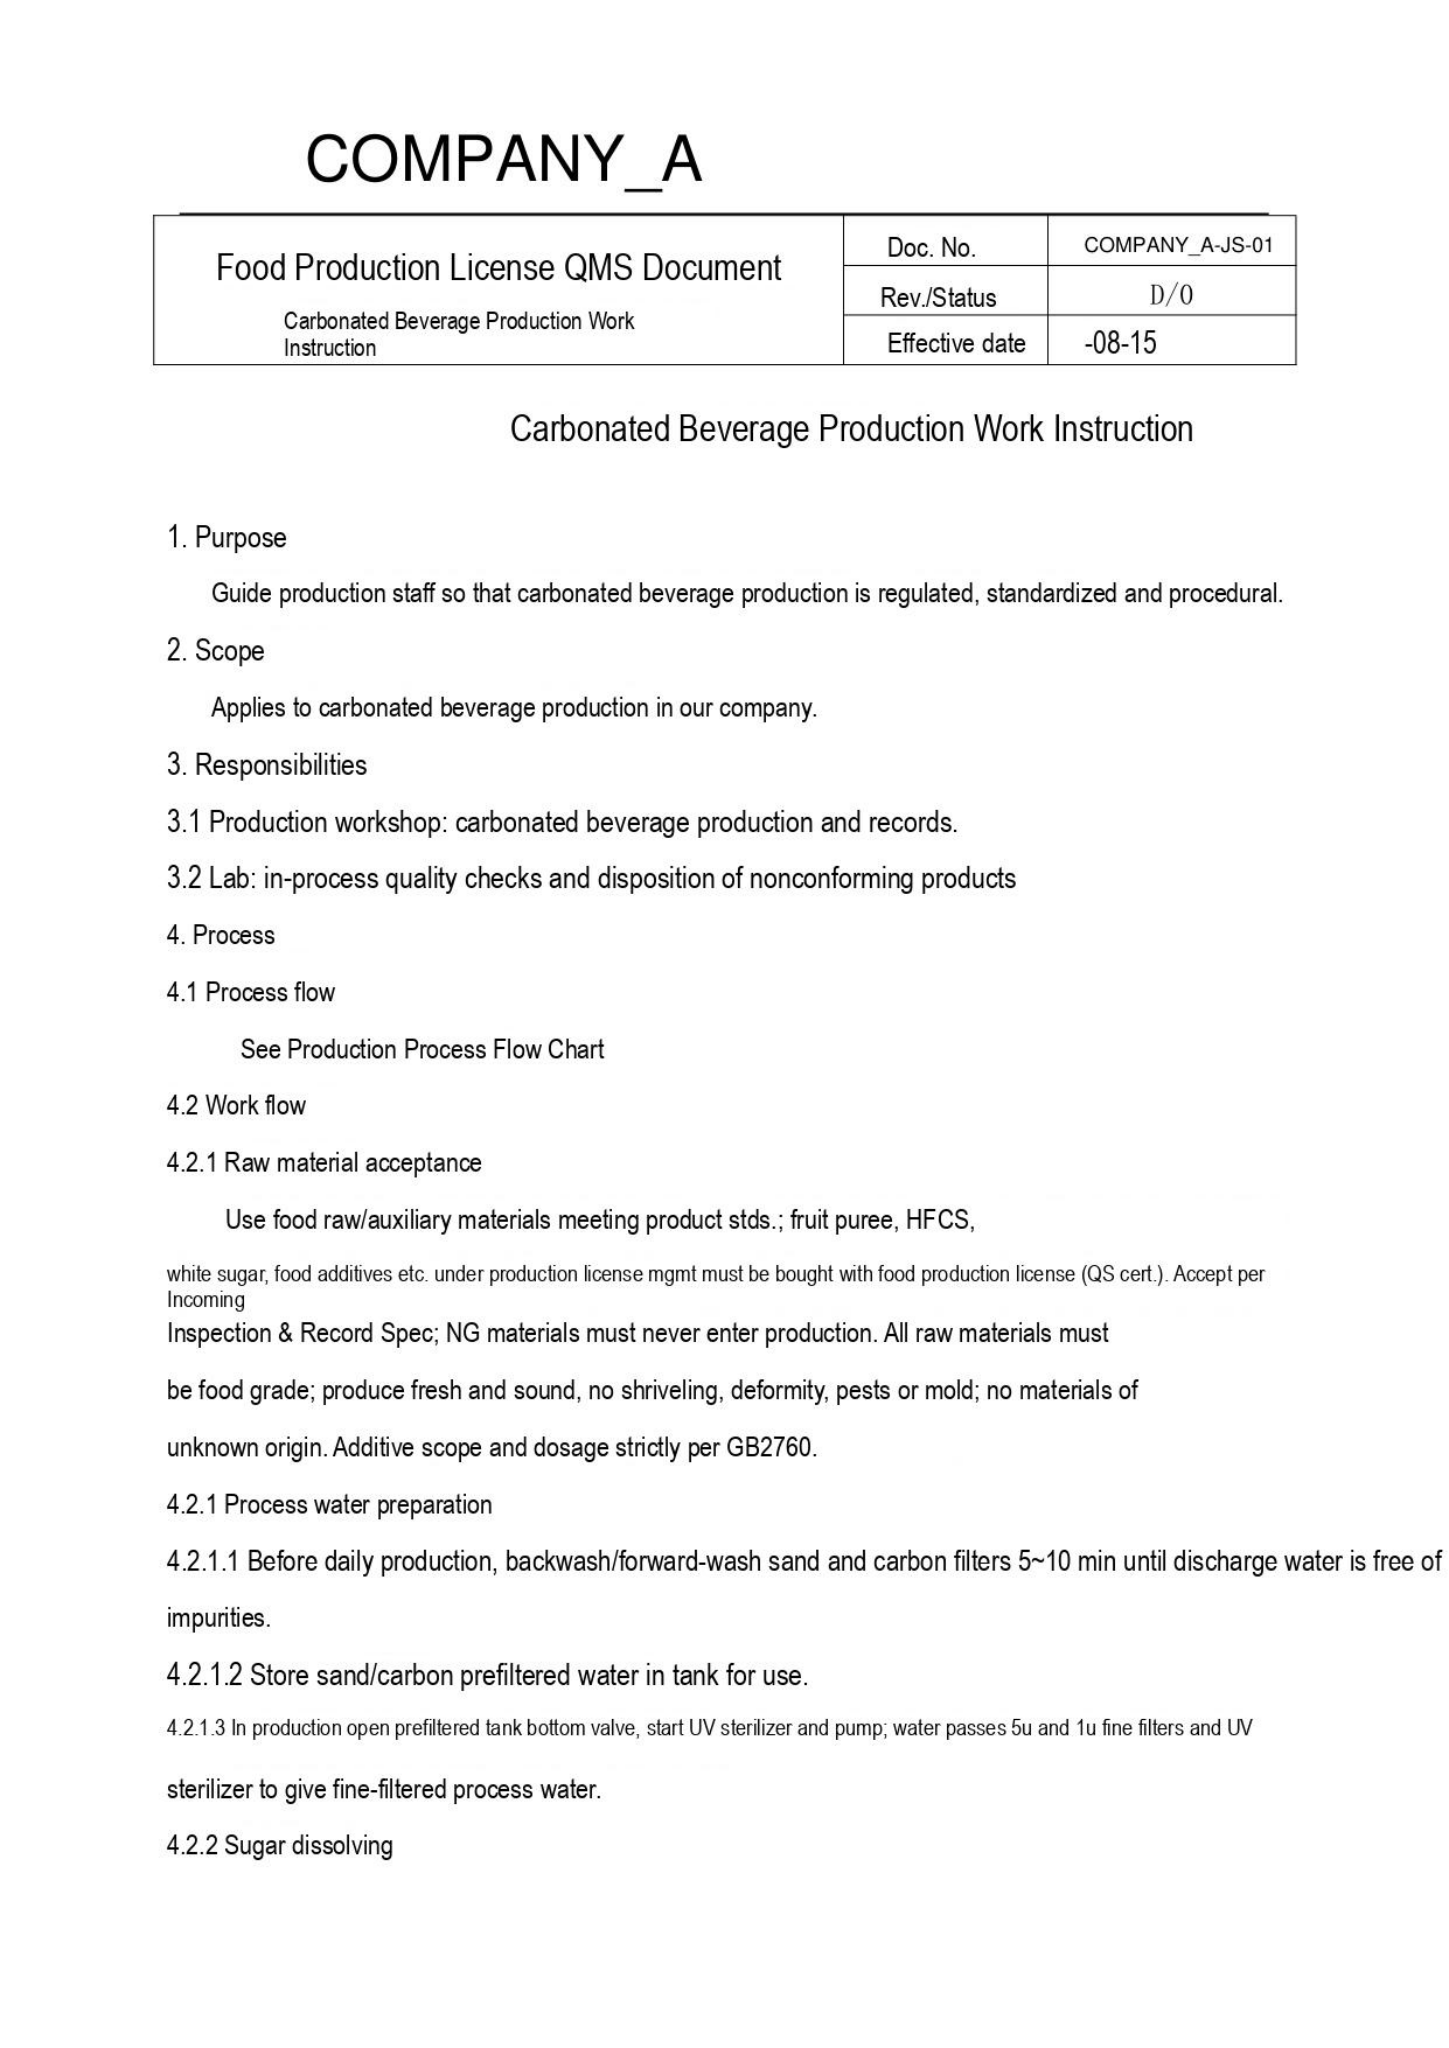COMPANY_A

| Food Production License QMS Document<br>Carbonated Beverage Production Work Instruction | Doc. No. | COMPANY_A-JS-01 |
|---|---|---|
| | Rev./Status | D/0 |
| | Effective date | -08-15 |

Carbonated Beverage Production Work Instruction

1. Purpose

Guide production staff so that carbonated beverage production is regulated, standardized and procedural.

2. Scope

Applies to carbonated beverage production in our company.

3. Responsibilities

3.1 Production workshop: carbonated beverage production and records.

3.2 Lab: in-process quality checks and disposition of nonconforming products

4. Process

4.1 Process flow

See Production Process Flow Chart

4.2 Work flow

4.2.1 Raw material acceptance

Use food raw/auxiliary materials meeting product stds.; fruit puree, HFCS,

white sugar, food additives etc. under production license mgmt must be bought with food production license (QS cert.). Accept per Incoming

Inspection & Record Spec; NG materials must never enter production. All raw materials must

be food grade; produce fresh and sound, no shriveling, deformity, pests or mold; no materials of

unknown origin. Additive scope and dosage strictly per GB2760.

4.2.1 Process water preparation

4.2.1.1 Before daily production, backwash/forward-wash sand and carbon filters 5~10 min until discharge water is free of impurities.

4.2.1.2 Store sand/carbon prefiltered water in tank for use.

4.2.1.3 In production open prefiltered tank bottom valve, start UV sterilizer and pump; water passes 5u and 1u fine filters and UV

sterilizer to give fine-filtered process water.

4.2.2 Sugar dissolving
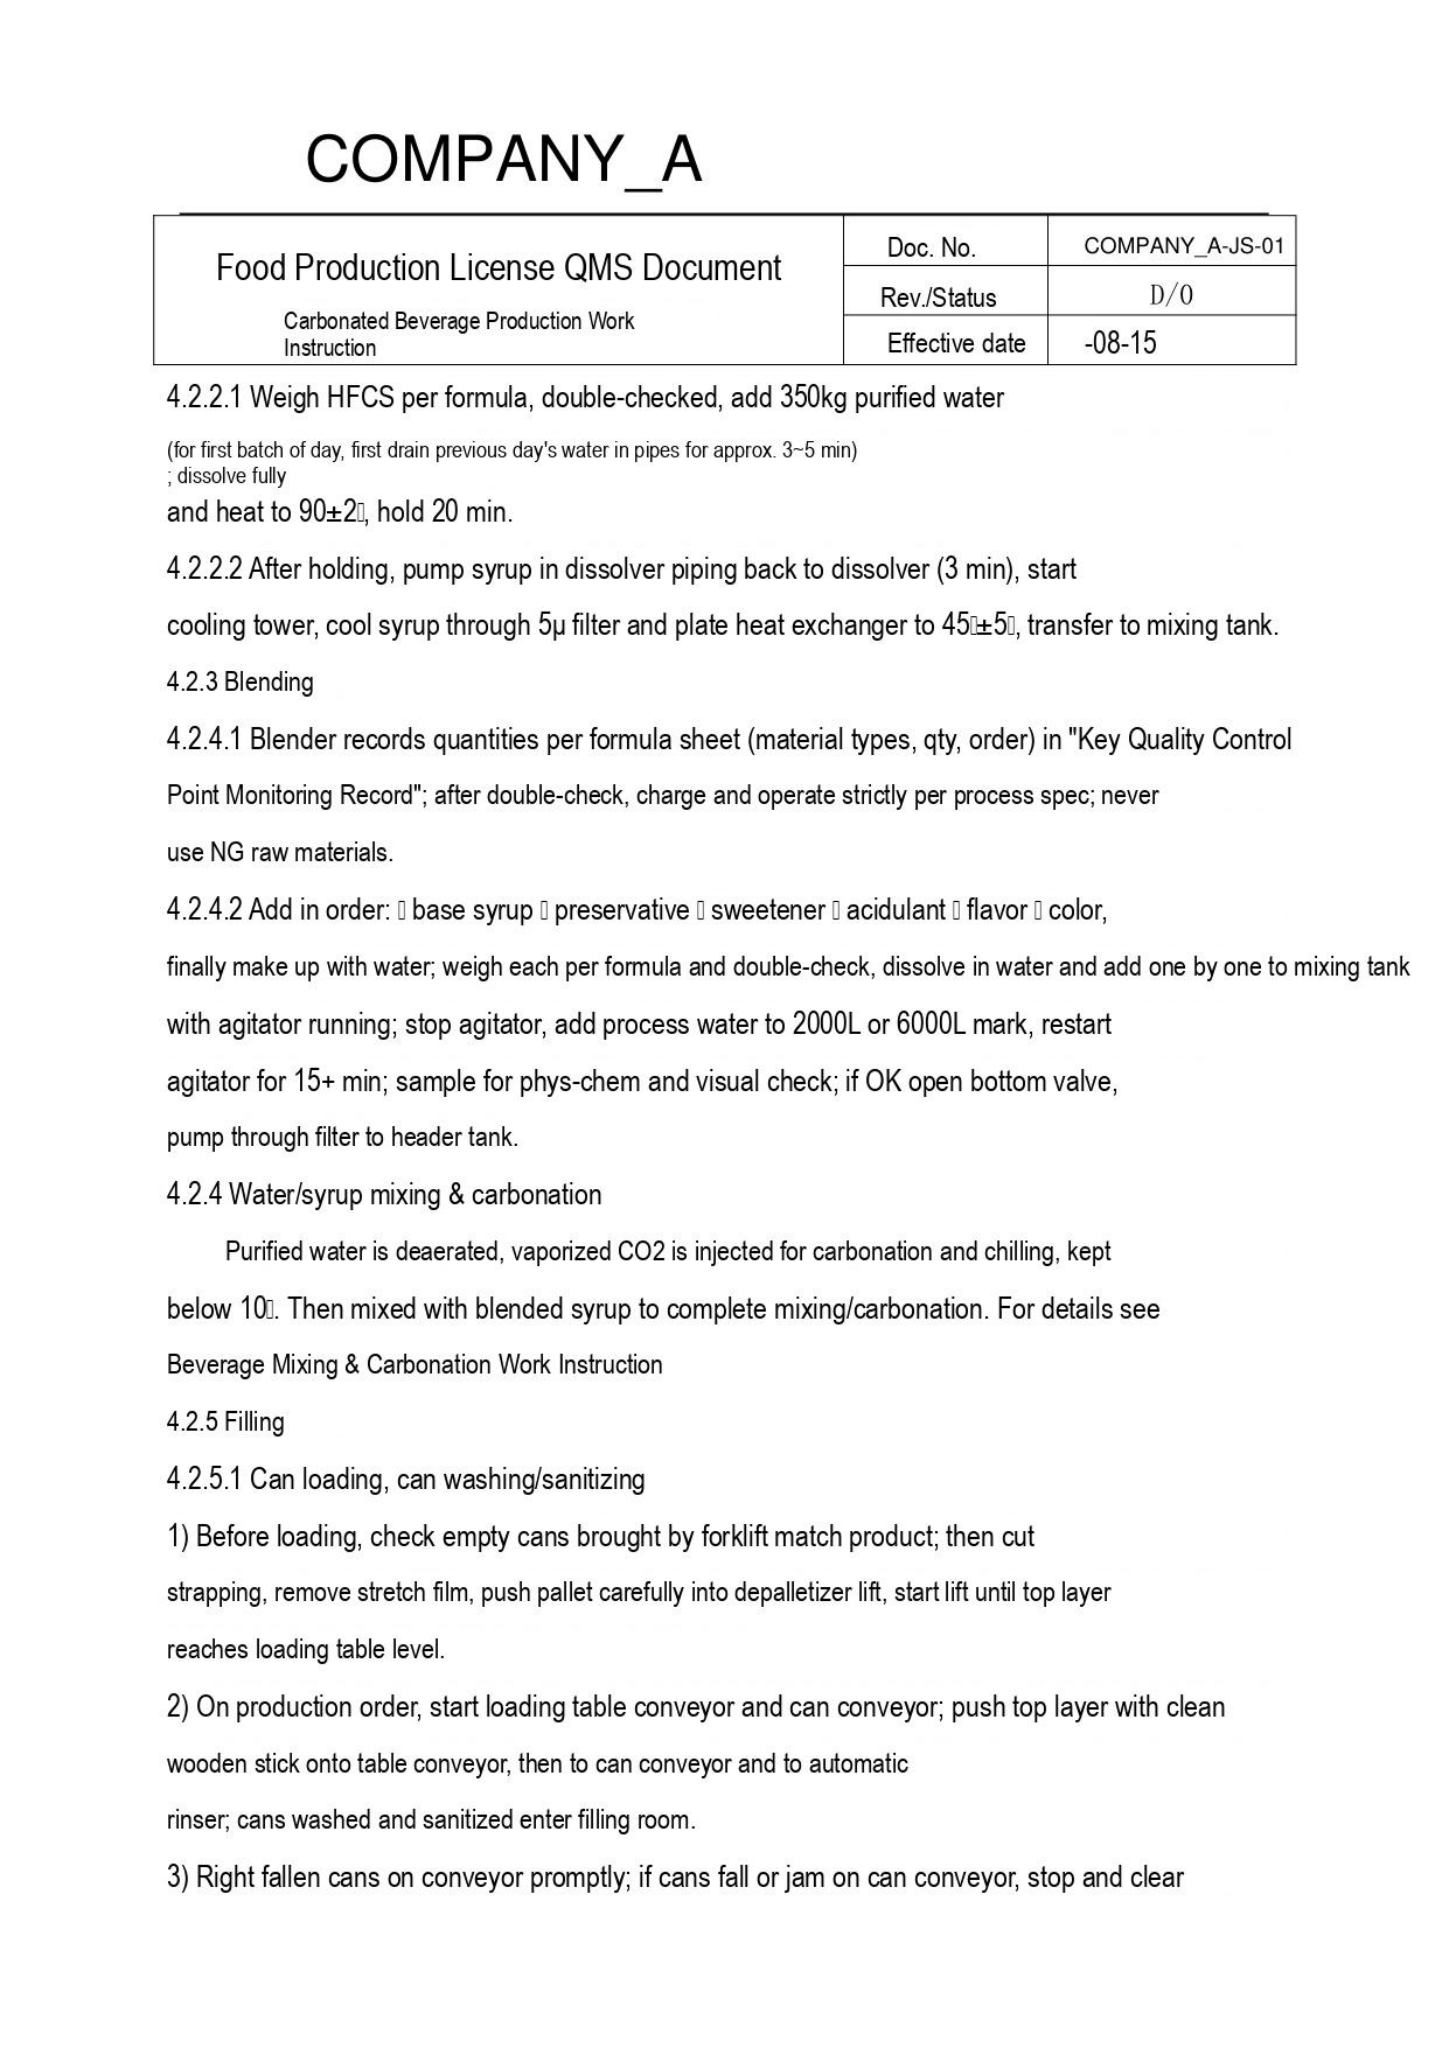COMPANY_A

| Food Production License QMS Document<br>Carbonated Beverage Production Work Instruction | Doc. No. | COMPANY_A-JS-01 |
|---|---|---|
| | Rev./Status | D/0 |
| | Effective date | -08-15 |

4.2.2.1 Weigh HFCS per formula, double-checked, add 350kg purified water

(for first batch of day, first drain previous day's water in pipes for approx. 3~5 min)
; dissolve fully

and heat to 90±2, hold 20 min.

4.2.2.2 After holding, pump syrup in dissolver piping back to dissolver (3 min), start

cooling tower, cool syrup through 5μ filter and plate heat exchanger to 45±5, transfer to mixing tank.

4.2.3 Blending

4.2.4.1 Blender records quantities per formula sheet (material types, qty, order) in "Key Quality Control

Point Monitoring Record"; after double-check, charge and operate strictly per process spec; never

use NG raw materials.

4.2.4.2 Add in order: base syrup preservative sweetener acidulant flavor color,

finally make up with water; weigh each per formula and double-check, dissolve in water and add one by one to mixing tank

with agitator running; stop agitator, add process water to 2000L or 6000L mark, restart

agitator for 15+ min; sample for phys-chem and visual check; if OK open bottom valve,

pump through filter to header tank.

4.2.4 Water/syrup mixing & carbonation

Purified water is deaerated, vaporized CO2 is injected for carbonation and chilling, kept

below 10. Then mixed with blended syrup to complete mixing/carbonation. For details see

Beverage Mixing & Carbonation Work Instruction

4.2.5 Filling

4.2.5.1 Can loading, can washing/sanitizing

1) Before loading, check empty cans brought by forklift match product; then cut

strapping, remove stretch film, push pallet carefully into depalletizer lift, start lift until top layer

reaches loading table level.

2) On production order, start loading table conveyor and can conveyor; push top layer with clean

wooden stick onto table conveyor, then to can conveyor and to automatic

rinser; cans washed and sanitized enter filling room.

3) Right fallen cans on conveyor promptly; if cans fall or jam on can conveyor, stop and clear
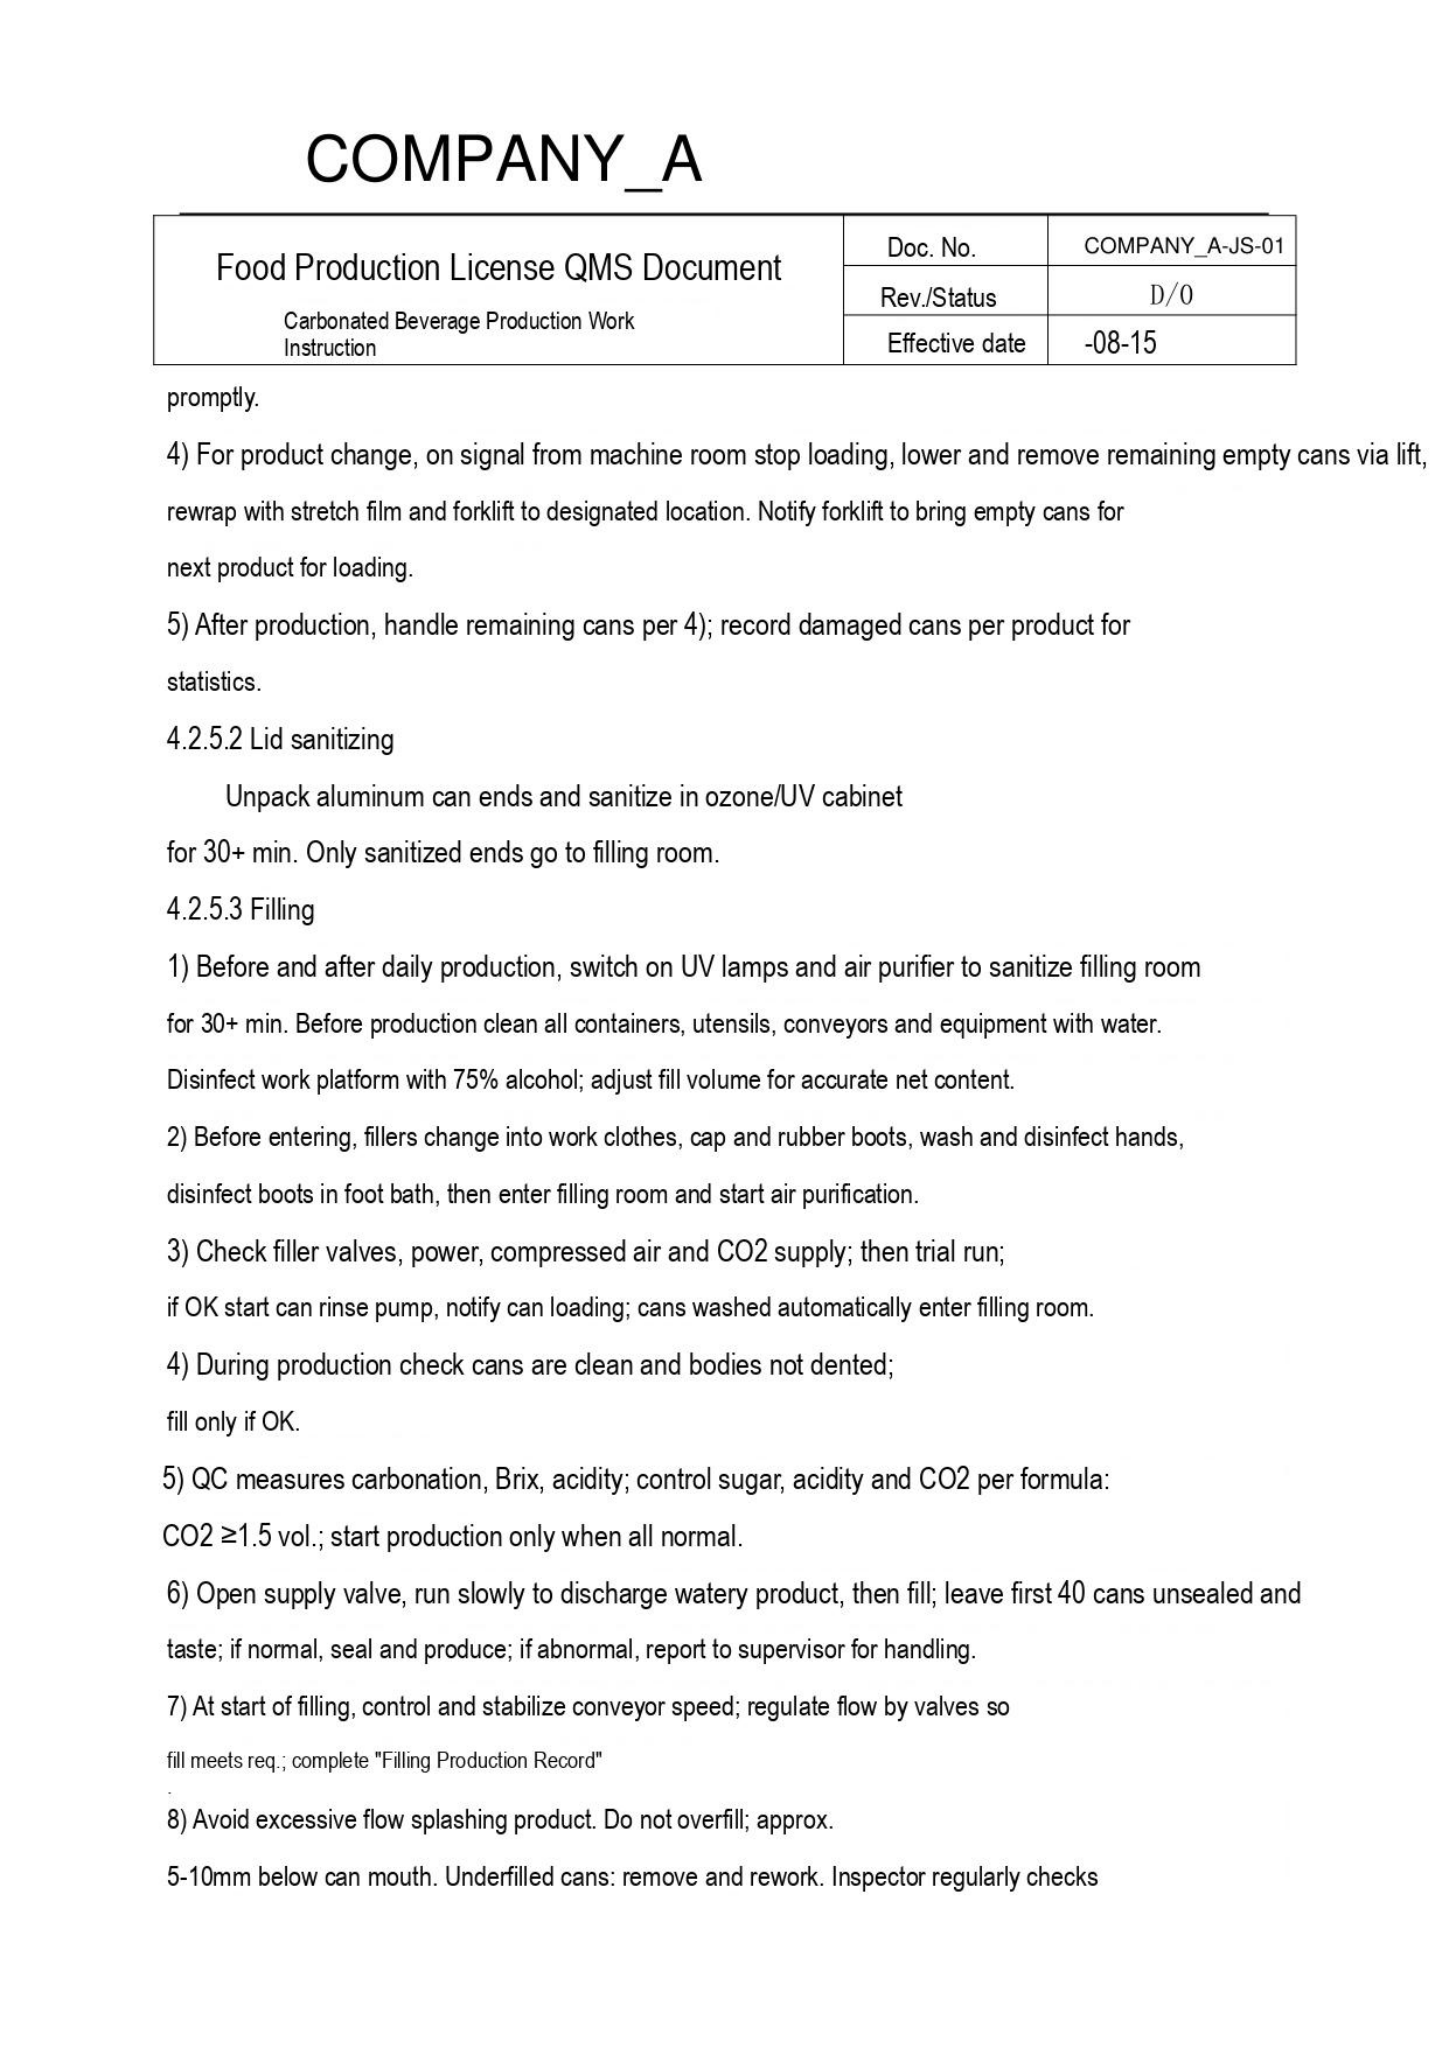COMPANY_A

| Food Production License QMS Document<br>Carbonated Beverage Production Work Instruction | Doc. No. | COMPANY_A-JS-01 |
|---|---|---|
| | Rev./Status | D/0 |
| | Effective date | -08-15 |

promptly.

4) For product change, on signal from machine room stop loading, lower and remove remaining empty cans via lift, rewrap with stretch film and forklift to designated location. Notify forklift to bring empty cans for next product for loading.

5) After production, handle remaining cans per 4); record damaged cans per product for statistics.

4.2.5.2 Lid sanitizing

Unpack aluminum can ends and sanitize in ozone/UV cabinet for 30+ min. Only sanitized ends go to filling room.

4.2.5.3 Filling

1) Before and after daily production, switch on UV lamps and air purifier to sanitize filling room for 30+ min. Before production clean all containers, utensils, conveyors and equipment with water. Disinfect work platform with 75% alcohol; adjust fill volume for accurate net content.

2) Before entering, fillers change into work clothes, cap and rubber boots, wash and disinfect hands, disinfect boots in foot bath, then enter filling room and start air purification.

3) Check filler valves, power, compressed air and CO2 supply; then trial run; if OK start can rinse pump, notify can loading; cans washed automatically enter filling room.

4) During production check cans are clean and bodies not dented; fill only if OK.

5) QC measures carbonation, Brix, acidity; control sugar, acidity and CO2 per formula: CO2 ≥1.5 vol.; start production only when all normal.

6) Open supply valve, run slowly to discharge watery product, then fill; leave first 40 cans unsealed and taste; if normal, seal and produce; if abnormal, report to supervisor for handling.

7) At start of filling, control and stabilize conveyor speed; regulate flow by valves so fill meets req.; complete "Filling Production Record"

8) Avoid excessive flow splashing product. Do not overfill; approx. 5-10mm below can mouth. Underfilled cans: remove and rework. Inspector regularly checks
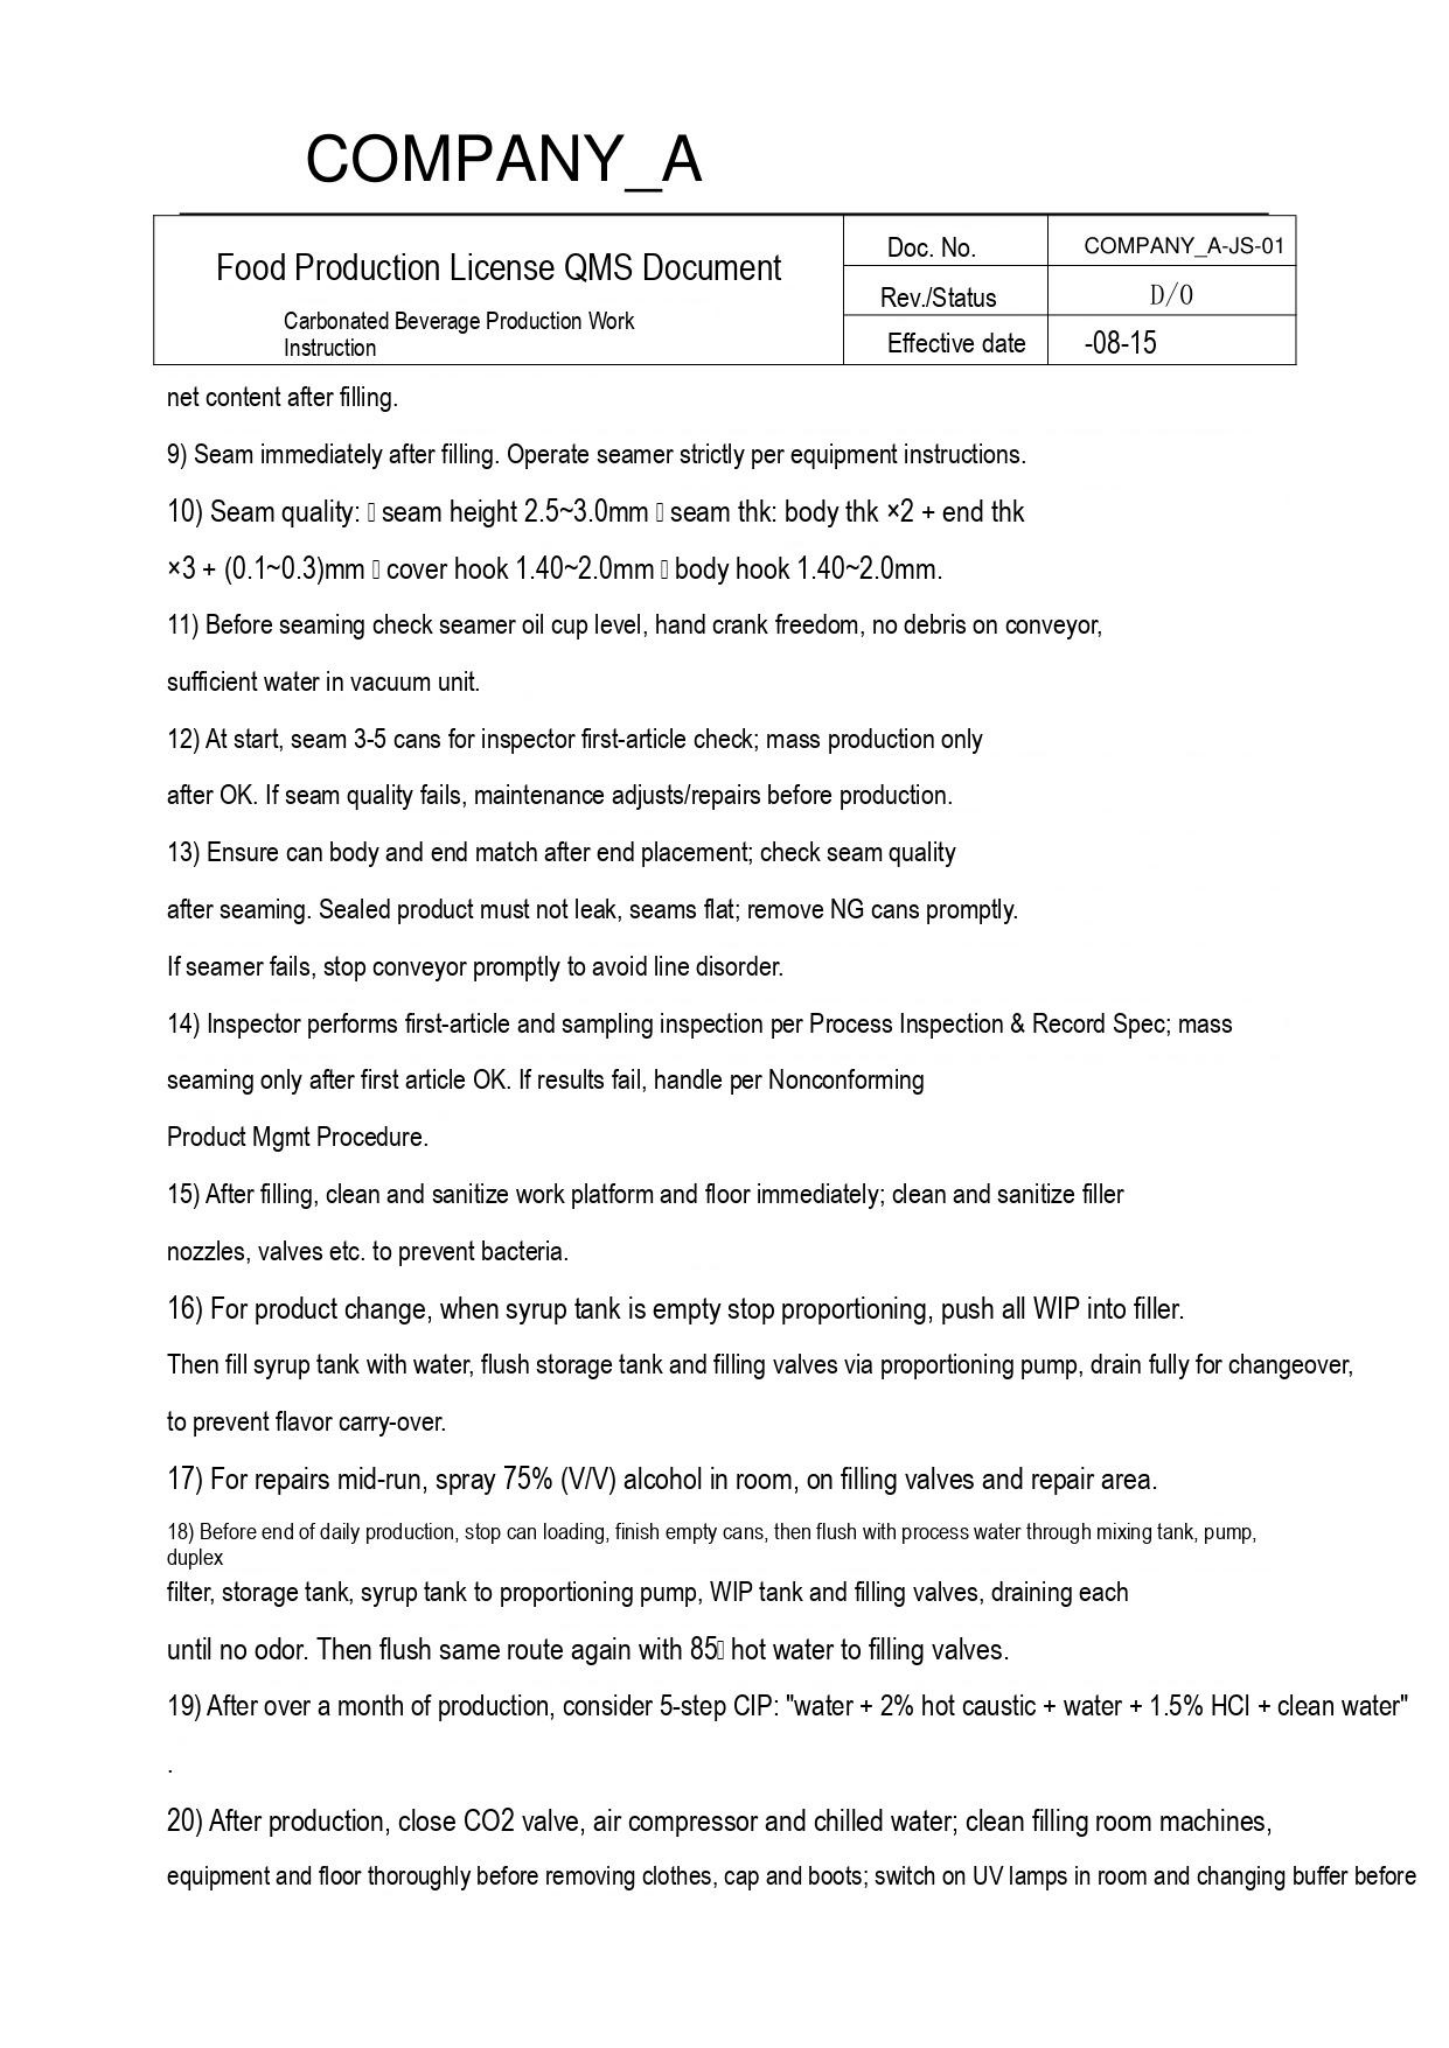COMPANY_A

| Food Production License QMS Document<br>Carbonated Beverage Production Work Instruction | Doc. No. | COMPANY_A-JS-01 |
|---|---|---|
| | Rev./Status | D/0 |
| | Effective date | -08-15 |

net content after filling.

9) Seam immediately after filling. Operate seamer strictly per equipment instructions.

10) Seam quality: seam height 2.5~3.0mm seam thk: body thk ×2 + end thk ×3 + (0.1~0.3)mm cover hook 1.40~2.0mm body hook 1.40~2.0mm.

11) Before seaming check seamer oil cup level, hand crank freedom, no debris on conveyor, sufficient water in vacuum unit.

12) At start, seam 3-5 cans for inspector first-article check; mass production only after OK. If seam quality fails, maintenance adjusts/repairs before production.

13) Ensure can body and end match after end placement; check seam quality after seaming. Sealed product must not leak, seams flat; remove NG cans promptly. If seamer fails, stop conveyor promptly to avoid line disorder.

14) Inspector performs first-article and sampling inspection per Process Inspection & Record Spec; mass seaming only after first article OK. If results fail, handle per Nonconforming Product Mgmt Procedure.

15) After filling, clean and sanitize work platform and floor immediately; clean and sanitize filler nozzles, valves etc. to prevent bacteria.

16) For product change, when syrup tank is empty stop proportioning, push all WIP into filler. Then fill syrup tank with water, flush storage tank and filling valves via proportioning pump, drain fully for changeover, to prevent flavor carry-over.

17) For repairs mid-run, spray 75% (V/V) alcohol in room, on filling valves and repair area.

18) Before end of daily production, stop can loading, finish empty cans, then flush with process water through mixing tank, pump, duplex filter, storage tank, syrup tank to proportioning pump, WIP tank and filling valves, draining each until no odor. Then flush same route again with 85 hot water to filling valves.

19) After over a month of production, consider 5-step CIP: "water + 2% hot caustic + water + 1.5% HCl + clean water".

20) After production, close CO2 valve, air compressor and chilled water; clean filling room machines, equipment and floor thoroughly before removing clothes, cap and boots; switch on UV lamps in room and changing buffer before
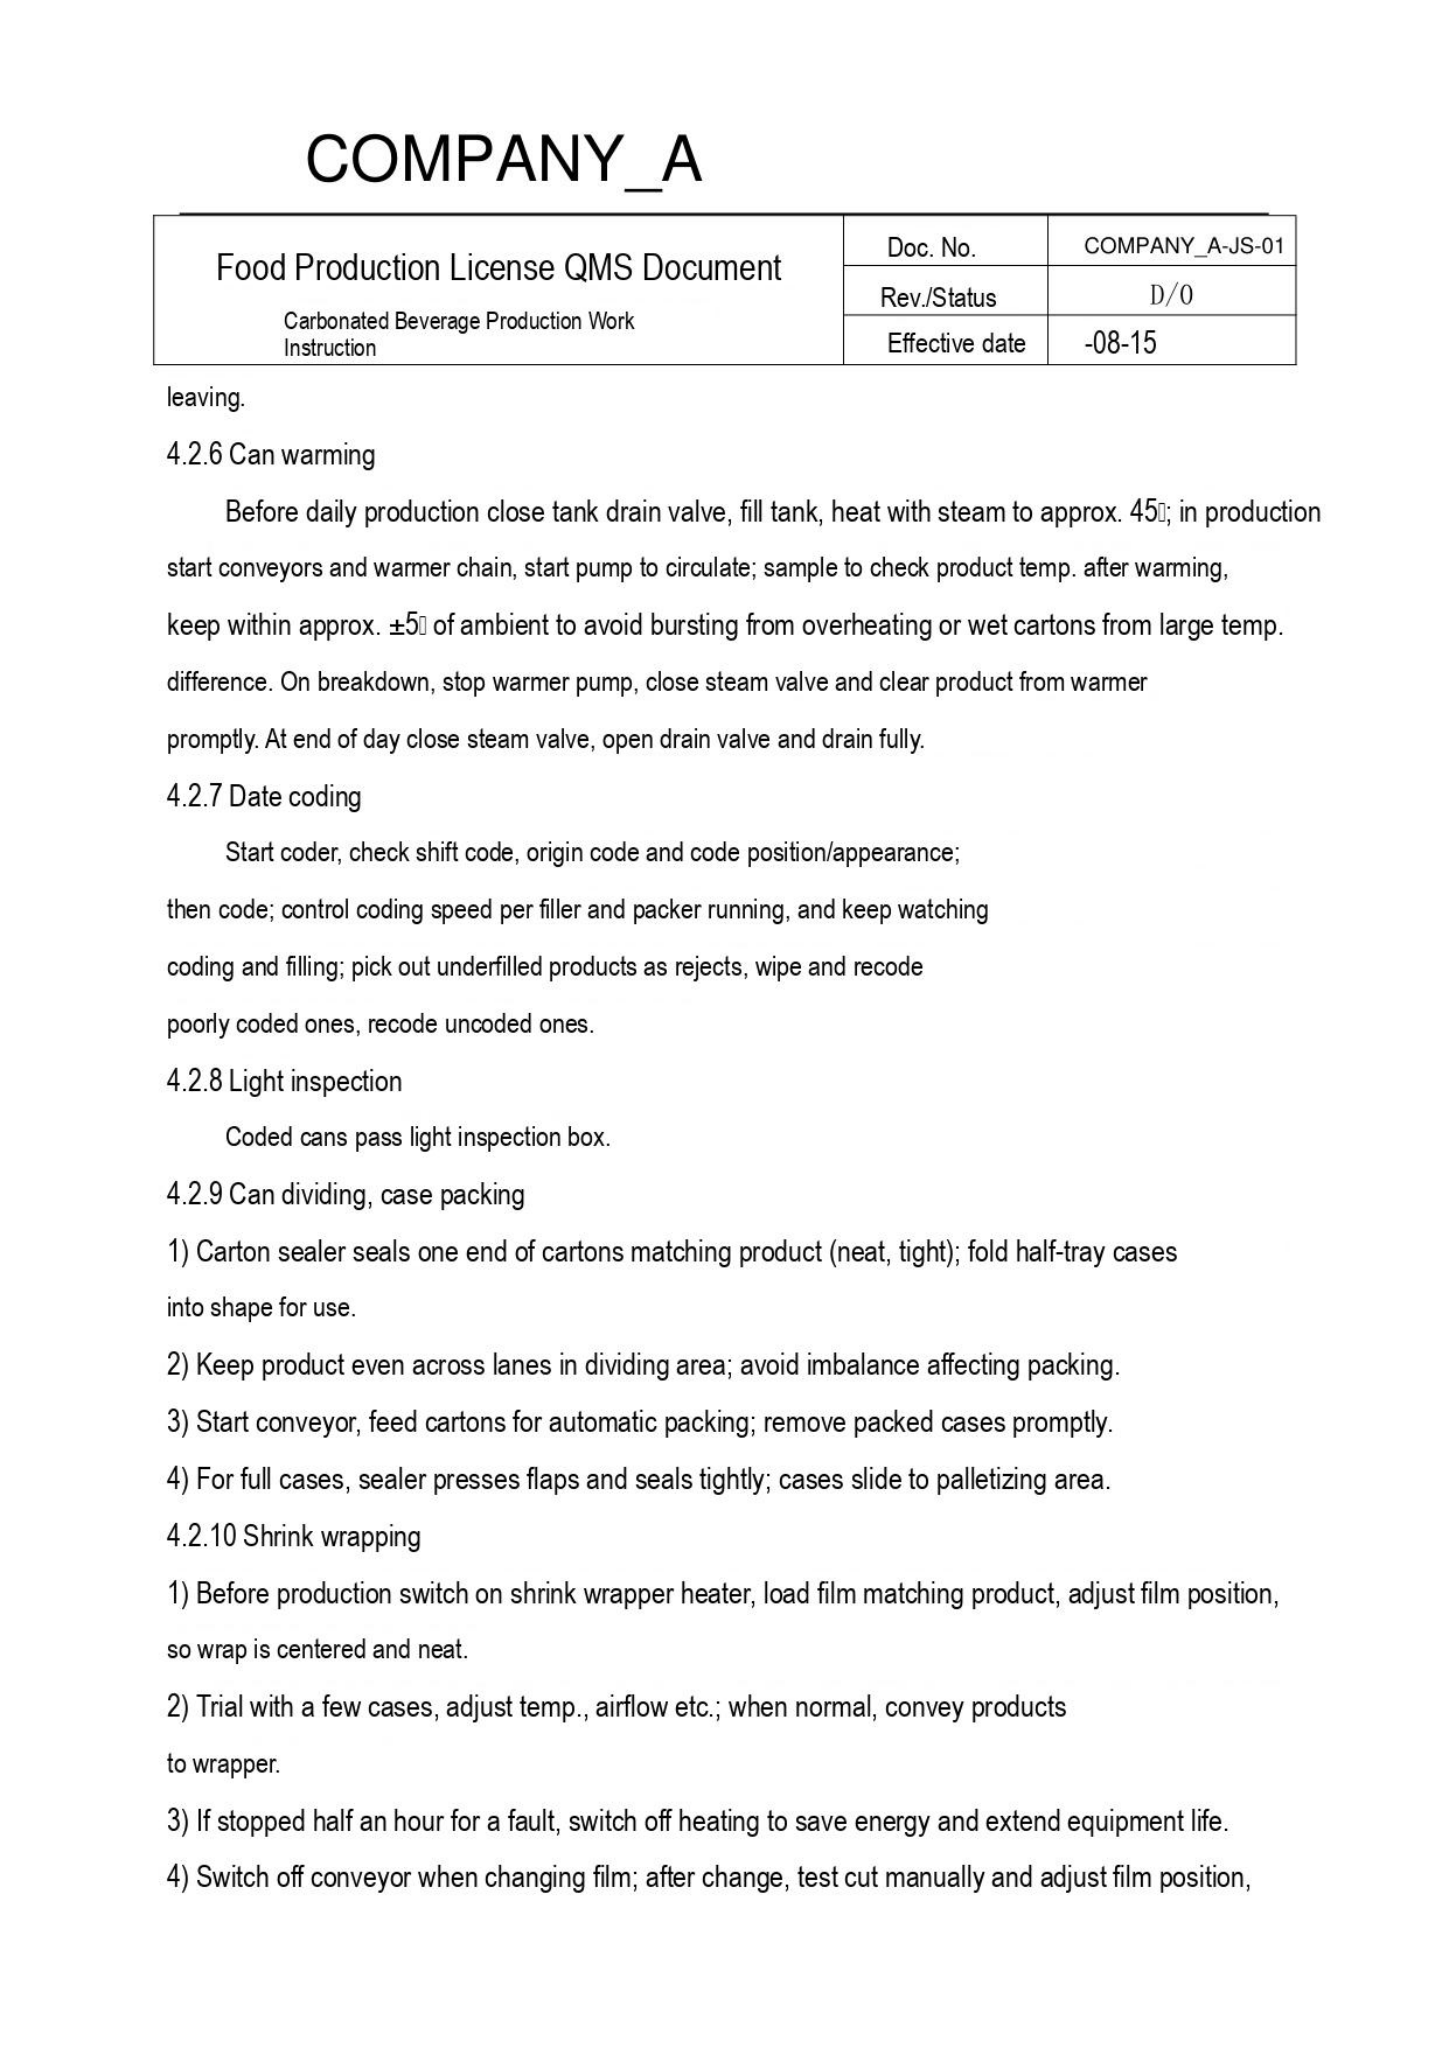COMPANY_A

| Food Production License QMS Document<br>Carbonated Beverage Production Work Instruction | Doc. No. | COMPANY_A-JS-01 |
|---|---|---|
| | Rev./Status | D/0 |
| | Effective date | -08-15 |

leaving.

4.2.6 Can warming

Before daily production close tank drain valve, fill tank, heat with steam to approx. 45; in production start conveyors and warmer chain, start pump to circulate; sample to check product temp. after warming, keep within approx. ±5 of ambient to avoid bursting from overheating or wet cartons from large temp. difference. On breakdown, stop warmer pump, close steam valve and clear product from warmer promptly. At end of day close steam valve, open drain valve and drain fully.

4.2.7 Date coding

Start coder, check shift code, origin code and code position/appearance; then code; control coding speed per filler and packer running, and keep watching coding and filling; pick out underfilled products as rejects, wipe and recode poorly coded ones, recode uncoded ones.

4.2.8 Light inspection

Coded cans pass light inspection box.

4.2.9 Can dividing, case packing

1) Carton sealer seals one end of cartons matching product (neat, tight); fold half-tray cases into shape for use.

2) Keep product even across lanes in dividing area; avoid imbalance affecting packing.

3) Start conveyor, feed cartons for automatic packing; remove packed cases promptly.

4) For full cases, sealer presses flaps and seals tightly; cases slide to palletizing area.

4.2.10 Shrink wrapping

1) Before production switch on shrink wrapper heater, load film matching product, adjust film position, so wrap is centered and neat.

2) Trial with a few cases, adjust temp., airflow etc.; when normal, convey products to wrapper.

3) If stopped half an hour for a fault, switch off heating to save energy and extend equipment life.

4) Switch off conveyor when changing film; after change, test cut manually and adjust film position,
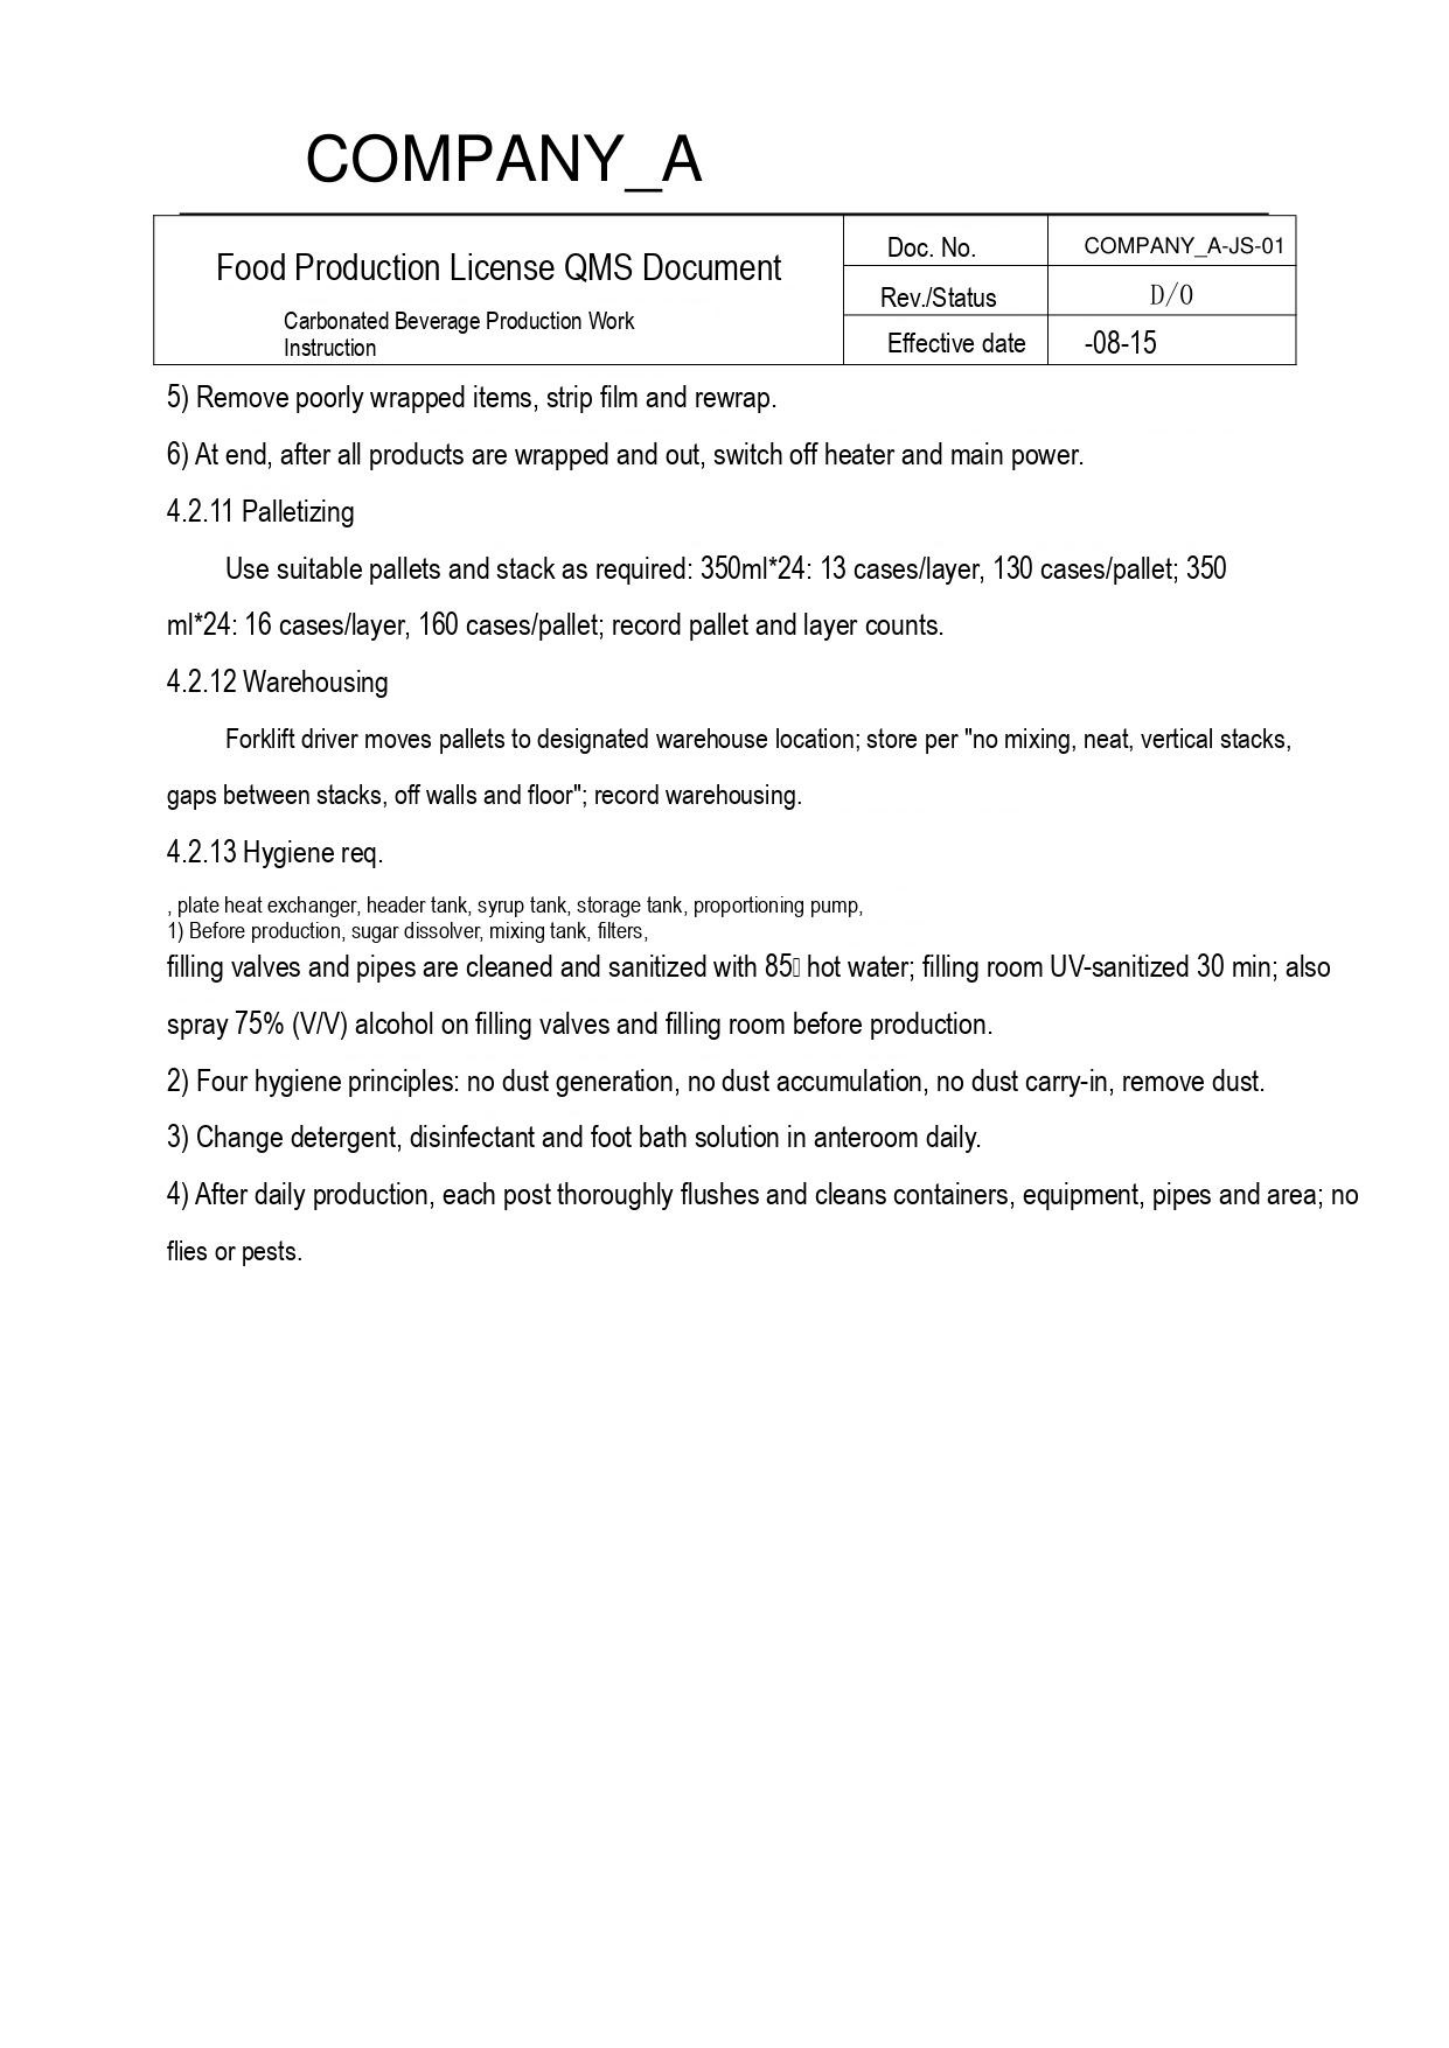COMPANY_A

| Food Production License QMS Document<br>Carbonated Beverage Production Work Instruction | Doc. No. | COMPANY_A-JS-01 |
|---|---|---|
| | Rev./Status | D/0 |
| | Effective date | -08-15 |

5) Remove poorly wrapped items, strip film and rewrap.

6) At end, after all products are wrapped and out, switch off heater and main power.

4.2.11 Palletizing

Use suitable pallets and stack as required: 350ml*24: 13 cases/layer, 130 cases/pallet; 350 ml*24: 16 cases/layer, 160 cases/pallet; record pallet and layer counts.

4.2.12 Warehousing

Forklift driver moves pallets to designated warehouse location; store per "no mixing, neat, vertical stacks, gaps between stacks, off walls and floor"; record warehousing.

4.2.13 Hygiene req.

, plate heat exchanger, header tank, syrup tank, storage tank, proportioning pump,
1) Before production, sugar dissolver, mixing tank, filters,
filling valves and pipes are cleaned and sanitized with 85 hot water; filling room UV-sanitized 30 min; also spray 75% (V/V) alcohol on filling valves and filling room before production.

2) Four hygiene principles: no dust generation, no dust accumulation, no dust carry-in, remove dust.

3) Change detergent, disinfectant and foot bath solution in anteroom daily.

4) After daily production, each post thoroughly flushes and cleans containers, equipment, pipes and area; no flies or pests.
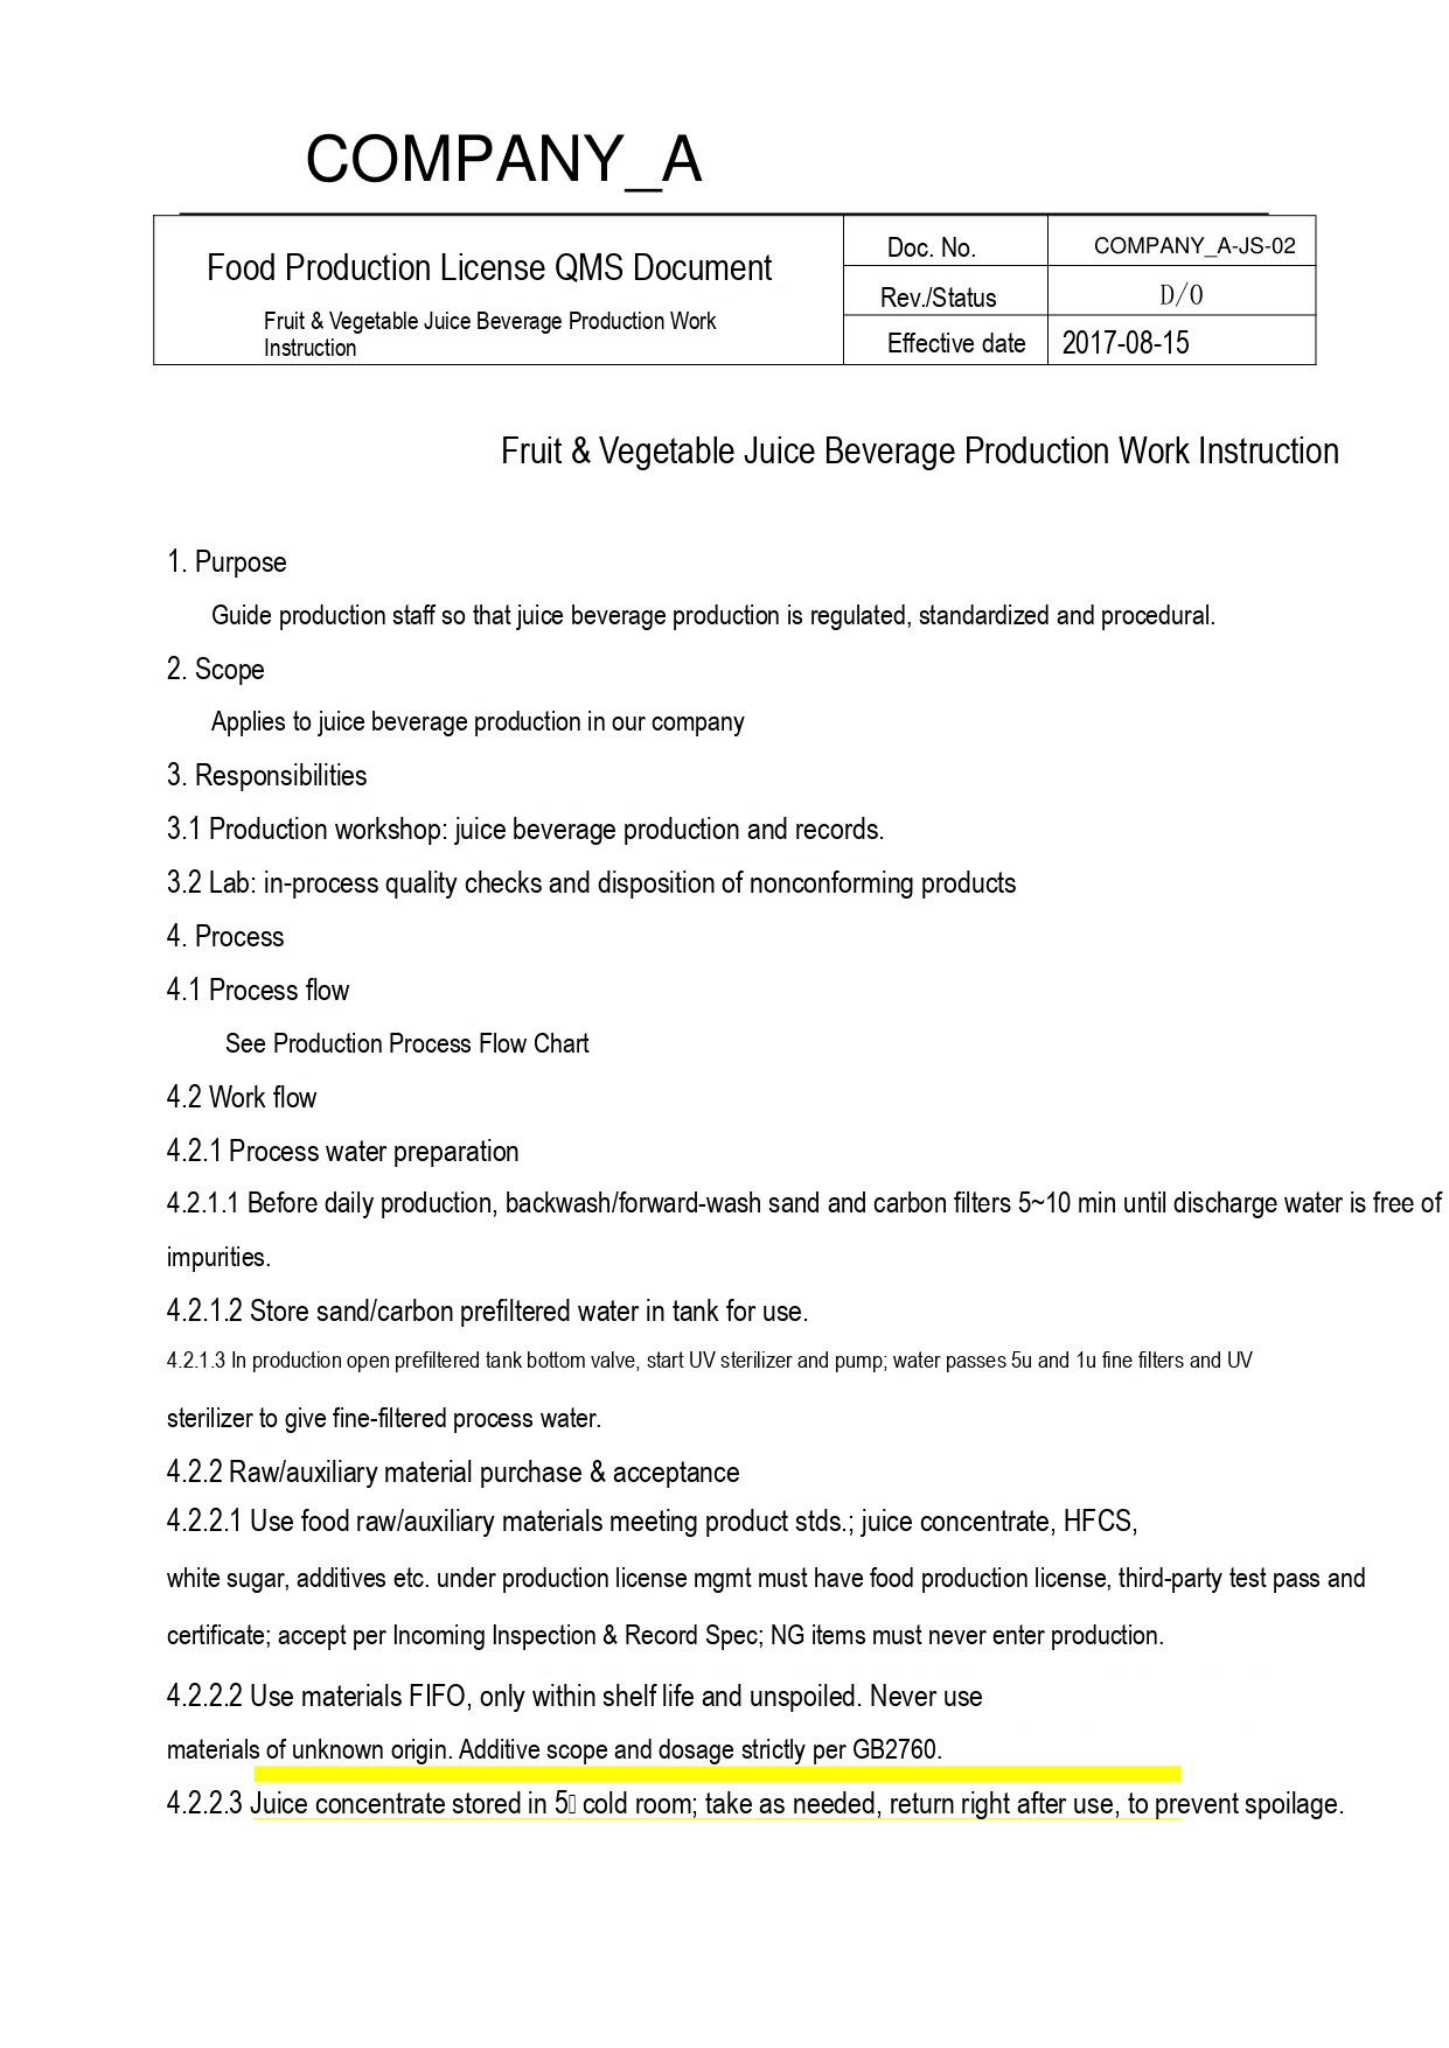COMPANY_A

| Food Production License QMS Document<br>Fruit & Vegetable Juice Beverage Production Work Instruction | Doc. No. | COMPANY_A-JS-02 |
|---|---|---|
| | Rev./Status | D/0 |
| | Effective date | 2017-08-15 |

Fruit & Vegetable Juice Beverage Production Work Instruction

1. Purpose

Guide production staff so that juice beverage production is regulated, standardized and procedural.

2. Scope

Applies to juice beverage production in our company

3. Responsibilities

3.1 Production workshop: juice beverage production and records.

3.2 Lab: in-process quality checks and disposition of nonconforming products

4. Process

4.1 Process flow

See Production Process Flow Chart

4.2 Work flow

4.2.1 Process water preparation

4.2.1.1 Before daily production, backwash/forward-wash sand and carbon filters 5~10 min until discharge water is free of impurities.

4.2.1.2 Store sand/carbon prefiltered water in tank for use.

4.2.1.3 In production open prefiltered tank bottom valve, start UV sterilizer and pump; water passes 5u and 1u fine filters and UV sterilizer to give fine-filtered process water.

4.2.2 Raw/auxiliary material purchase & acceptance

4.2.2.1 Use food raw/auxiliary materials meeting product stds.; juice concentrate, HFCS, white sugar, additives etc. under production license mgmt must have food production license, third-party test pass and certificate; accept per Incoming Inspection & Record Spec; NG items must never enter production.

4.2.2.2 Use materials FIFO, only within shelf life and unspoiled. Never use materials of unknown origin. Additive scope and dosage strictly per GB2760.

4.2.2.3 Juice concentrate stored in 5 cold room; take as needed, return right after use, to prevent spoilage.